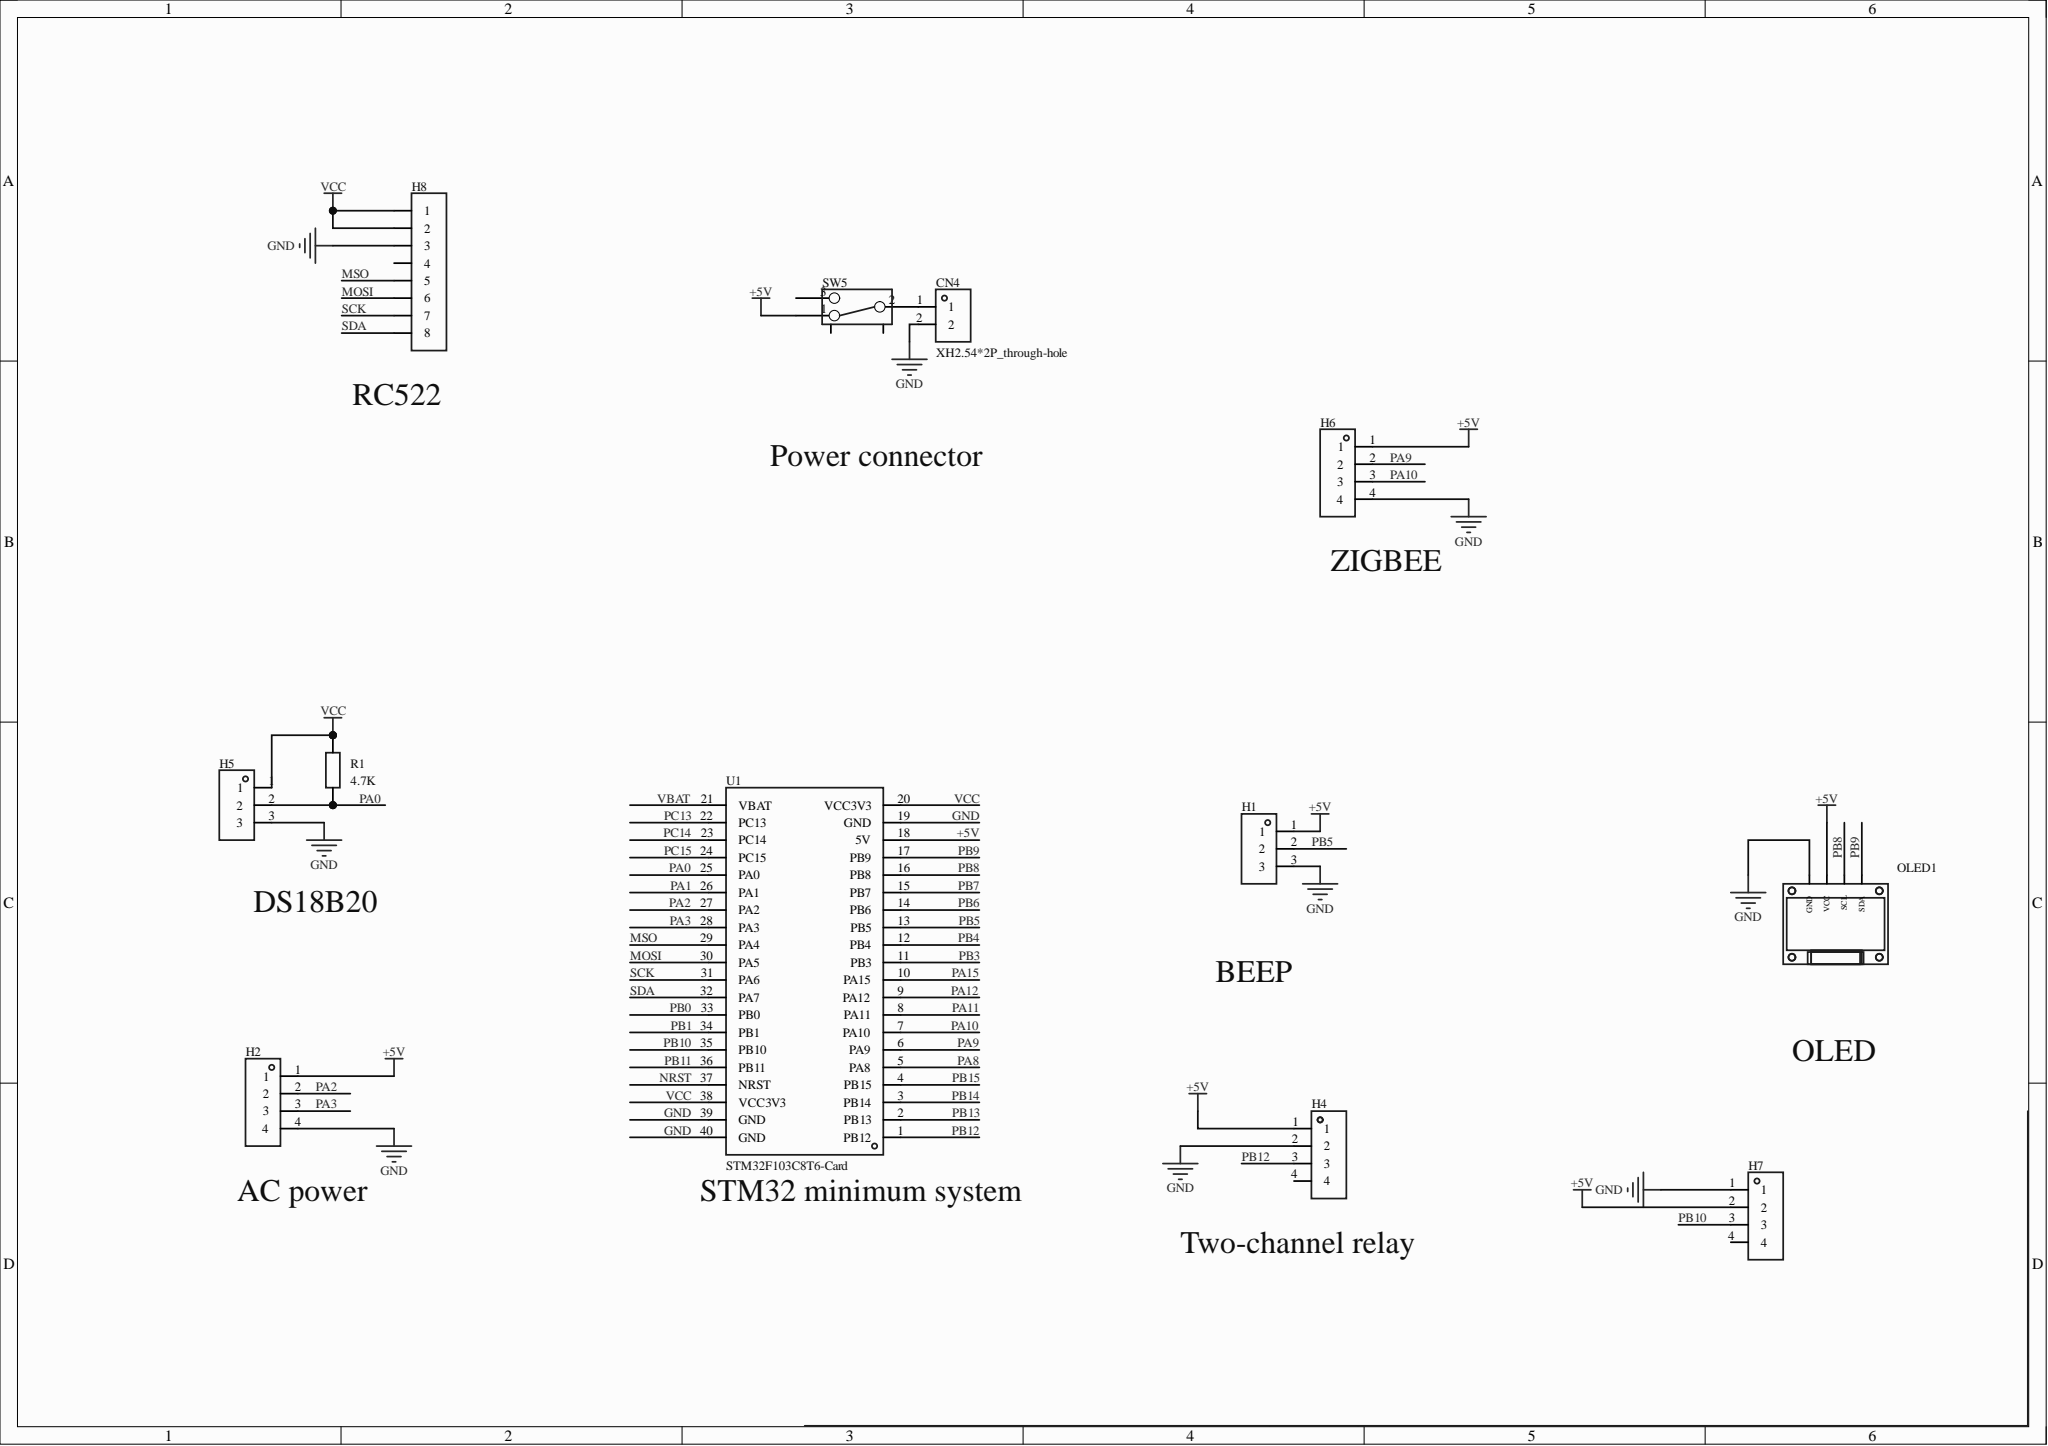Circuit board | Altium Designer | 12 parts | 18 nets
Bill of materials:
Comment,Description,Designator,Footprint,LibRef,Quantity
"XH2.54*2P_through-hole","","CN4","CONN-TH_2P-P2.50-XH2.54-2P","XH2.54*2P_直插","1"
"","","H1, H5","HDR-TH_3P-P2.54-V-F","HDR-F_2.54_1x3P","2"
"","","H2, H4, H6","HDR-TH_4P-P2.54-V-F","HDR-F_2.54_1x4P","3"
"","","H7","HDR-TH_4P-P2.54-V-M","HDR-M_2.54_1x4P","1"
"","","H8","HDR-TH_8P-P2.54-V-F-1","HDR-F_2.54_1x8P","1"
"","","OLED1","0.96OLED_4P","0.96OLED模块_4P","1"
"4.7K","","R1","R0603","Res_0603","1"
"","","SW5","拨动开关","拨动开关_正","1"
"STM32F103C8T6-Card","","U1","CONN-TH_L53.3-W22.9_STM32F103C8T6-CARD","STM32F103C8T6-Card","1"
Netlist (Protel format):
[
CN4
CONN-TH_2P-P2.50-XH2.54-2P
XH2.54*2P_through-hole



]
[
H1
HDR-TH_3P-P2.54-V-F




]
[
H2
HDR-TH_4P-P2.54-V-F




]
[
H4
HDR-TH_4P-P2.54-V-F




]
[
H5
HDR-TH_3P-P2.54-V-F




]
[
H6
HDR-TH_4P-P2.54-V-F




]
[
H7
HDR-TH_4P-P2.54-V-M




]
[
H8
HDR-TH_8P-P2.54-V-F-1




]
[
OLED1
0.96OLED_4P




]
[
R1
R0603
4.7K



]
[
SW5
拨动开关




]
[
U1
CONN-TH_L53.3-W22.9_STM32F103C8T6-CARD
STM32F103C8T6-Card



]
(
VCC
H5-1
H8-1
H8-2
R1-2
U1-20
U1-38
)
(
SDA
H8-8
U1-32
)
(
SCK
H8-7
U1-31
)
(
PB12
H4-3
U1-1
)
(
PB10
H7-3
U1-35
)
(
PB9
OLED1-4
U1-17
)
(
PB8
OLED1-3
U1-16
)
(
PB5
H1-2
U1-13
)
(
PA10
H6-3
U1-7
)
(
PA9
H6-2
U1-6
)
(
PA3
H2-3
U1-28
)
(
PA2
H2-2
U1-27
)
(
PA0
H5-2
R1-1
U1-25
)
(
NetCN4_1
CN4-1
SW5-2
)
(
MSO
H8-5
U1-29
)
(
MOSI
H8-6
U1-30
)
(
GND
CN4-2
H1-3
H2-4
H4-2
H5-3
H6-4
H7-1
H8-3
OLED1-1
U1-19
U1-39
U1-40
)
(
+5V
H1-1
H2-1
H4-1
H6-1
H7-2
OLED1-2
SW5-1
U1-18
)